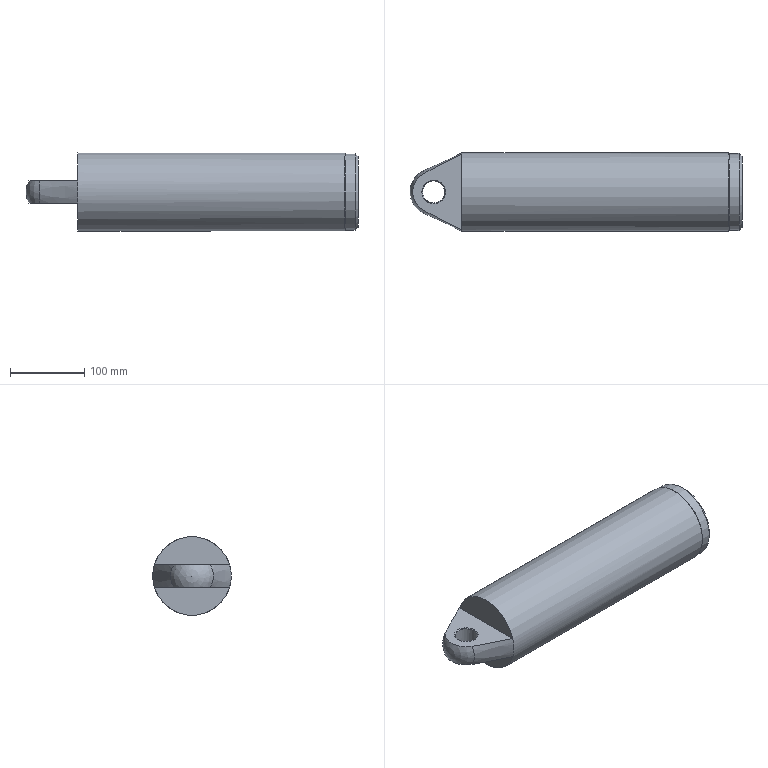Part | NX | features 侧推千斤顶缸 2 | 1 solid | 17 faces | box 448 x 106 x 106 mm | volume 2799935 mm3 | cone 6 | plane 6 | cylinder 4 | sphere 1 | commonest cylinder face diameters 30 x1 50.16 x1 104 x1 106 x1
STEP:
#1=CARTESIAN_POINT('',(0.,-50.833,-15.));
#2=VERTEX_POINT('',#1);
#3=CARTESIAN_POINT('',(0.,-50.833,15.));
#4=VERTEX_POINT('',#3);
#5=CARTESIAN_POINT('',(0.,0.,0.));
#6=DIRECTION('',(-1.,0.,0.));
#7=DIRECTION('',(0.,-1.,0.));
#8=AXIS2_PLACEMENT_3D('',#5,#6,#7);
#9=CIRCLE('',#8,53.);
#10=EDGE_CURVE('',#2,#4,#9,.T.);
#11=ORIENTED_EDGE('',*,*,#10,.T.);
#12=CARTESIAN_POINT('',(-51.511,-24.829,15.));
#13=VERTEX_POINT('',#12);
#14=CARTESIAN_POINT('',(0.,-50.833,15.));
#15=CARTESIAN_POINT('',(-8.652,-46.632,15.));
#16=CARTESIAN_POINT('',(-25.92,-38.162,15.));
#17=CARTESIAN_POINT('',(-43.068,-29.423,15.));
#18=CARTESIAN_POINT('',(-51.511,-24.829,15.));
#19=B_SPLINE_CURVE_WITH_KNOTS('',3,(#14,#15,#16,#17,#18),.UNSPECIFIED.,.F.,.F.,(4,1,4),(0.07837,0.1072,0.1361),.UNSPECIFIED.);
#20=EDGE_CURVE('',#4,#13,#19,.T.);
#21=ORIENTED_EDGE('',*,*,#20,.T.);
#22=CARTESIAN_POINT('',(-51.511,-24.829,-15.));
#23=VERTEX_POINT('',#22);
#24=CARTESIAN_POINT('',(-51.511,0.,0.));
#25=DIRECTION('',(-1.,0.,0.));
#26=DIRECTION('',(0.,-1.,0.));
#27=AXIS2_PLACEMENT_3D('',#24,#25,#26);
#28=CIRCLE('',#27,29.008);
#29=EDGE_CURVE('',#23,#13,#28,.T.);
#30=ORIENTED_EDGE('',*,*,#29,.F.);
#31=CARTESIAN_POINT('',(-51.511,-24.829,-15.));
#32=CARTESIAN_POINT('',(-43.068,-29.423,-15.));
#33=CARTESIAN_POINT('',(-25.924,-38.16,-15.));
#34=CARTESIAN_POINT('',(-8.652,-46.631,-15.));
#35=CARTESIAN_POINT('',(0.,-50.833,-15.));
#36=B_SPLINE_CURVE_WITH_KNOTS('',3,(#31,#32,#33,#34,#35),.UNSPECIFIED.,.F.,.F.,(4,1,4),(0.2163,0.2453,0.2742),.UNSPECIFIED.);
#37=EDGE_CURVE('',#23,#2,#36,.T.);
#38=ORIENTED_EDGE('',*,*,#37,.T.);
#39=EDGE_LOOP('',(#11,#21,#30,#38));
#40=FACE_BOUND('',#39,.T.);
#41=CARTESIAN_POINT('',(0.,0.,0.));
#42=DIRECTION('',(1.,0.,0.));
#43=DIRECTION('',(0.,1.,0.));
#44=AXIS2_PLACEMENT_3D('',#41,#42,#43);
#45=CONICAL_SURFACE('',#44,53.,0.4359);
#46=ADVANCED_FACE('',(#40),#45,.T.);
#47=CARTESIAN_POINT('',(-51.511,24.829,15.));
#48=VERTEX_POINT('',#47);
#49=CARTESIAN_POINT('',(-51.511,24.829,-15.));
#50=VERTEX_POINT('',#49);
#51=CARTESIAN_POINT('',(-51.511,0.,0.));
#52=DIRECTION('',(-1.,0.,0.));
#53=DIRECTION('',(0.,-1.,0.));
#54=AXIS2_PLACEMENT_3D('',#51,#52,#53);
#55=CIRCLE('',#54,29.008);
#56=EDGE_CURVE('',#48,#50,#55,.T.);
#57=ORIENTED_EDGE('',*,*,#56,.F.);
#58=CARTESIAN_POINT('',(0.,50.833,15.));
#59=VERTEX_POINT('',#58);
#60=CARTESIAN_POINT('',(-51.511,24.829,15.));
#61=CARTESIAN_POINT('',(-43.068,29.423,15.));
#62=CARTESIAN_POINT('',(-25.924,38.16,15.));
#63=CARTESIAN_POINT('',(-8.652,46.631,15.));
#64=CARTESIAN_POINT('',(0.,50.833,15.));
#65=B_SPLINE_CURVE_WITH_KNOTS('',3,(#60,#61,#62,#63,#64),.UNSPECIFIED.,.F.,.F.,(4,1,4),(0.2163,0.2453,0.2742),.UNSPECIFIED.);
#66=EDGE_CURVE('',#48,#59,#65,.T.);
#67=ORIENTED_EDGE('',*,*,#66,.T.);
#68=CARTESIAN_POINT('',(0.,50.833,-15.));
#69=VERTEX_POINT('',#68);
#70=CARTESIAN_POINT('',(0.,0.,0.));
#71=DIRECTION('',(-1.,0.,0.));
#72=DIRECTION('',(0.,-1.,0.));
#73=AXIS2_PLACEMENT_3D('',#70,#71,#72);
#74=CIRCLE('',#73,53.);
#75=EDGE_CURVE('',#59,#69,#74,.T.);
#76=ORIENTED_EDGE('',*,*,#75,.T.);
#77=CARTESIAN_POINT('',(0.,50.833,-15.));
#78=CARTESIAN_POINT('',(-8.652,46.632,-15.));
#79=CARTESIAN_POINT('',(-25.92,38.162,-15.));
#80=CARTESIAN_POINT('',(-43.068,29.423,-15.));
#81=CARTESIAN_POINT('',(-51.511,24.829,-15.));
#82=B_SPLINE_CURVE_WITH_KNOTS('',3,(#77,#78,#79,#80,#81),.UNSPECIFIED.,.F.,.F.,(4,1,4),(0.07837,0.1072,0.1361),.UNSPECIFIED.);
#83=EDGE_CURVE('',#69,#50,#82,.T.);
#84=ORIENTED_EDGE('',*,*,#83,.T.);
#85=EDGE_LOOP('',(#57,#67,#76,#84));
#86=FACE_BOUND('',#85,.T.);
#87=CARTESIAN_POINT('',(0.,0.,0.));
#88=DIRECTION('',(1.,0.,0.));
#89=DIRECTION('',(0.,1.,0.));
#90=AXIS2_PLACEMENT_3D('',#87,#88,#89);
#91=CONICAL_SURFACE('',#90,53.,0.4359);
#92=ADVANCED_FACE('',(#86),#91,.T.);
#93=ORIENTED_EDGE('',*,*,#29,.T.);
#94=CARTESIAN_POINT('',(-38.,0.,15.));
#95=DIRECTION('',(0.,0.,-1.));
#96=DIRECTION('',(0.,1.,0.));
#97=AXIS2_PLACEMENT_3D('',#94,#95,#96);
#98=CIRCLE('',#97,28.267);
#99=EDGE_CURVE('',#13,#48,#98,.T.);
#100=ORIENTED_EDGE('',*,*,#99,.T.);
#101=ORIENTED_EDGE('',*,*,#56,.T.);
#102=CARTESIAN_POINT('',(-38.,0.,-15.));
#103=DIRECTION('',(0.,0.,1.));
#104=DIRECTION('',(0.,-1.,0.));
#105=AXIS2_PLACEMENT_3D('',#102,#103,#104);
#106=CIRCLE('',#105,28.267);
#107=EDGE_CURVE('',#50,#23,#106,.T.);
#108=ORIENTED_EDGE('',*,*,#107,.T.);
#109=EDGE_LOOP('',(#93,#100,#101,#108));
#110=FACE_BOUND('',#109,.T.);
#111=CARTESIAN_POINT('',(-38.,0.,0.));
#112=DIRECTION('',(-1.,0.,0.));
#113=DIRECTION('',(0.,1.,0.));
#114=AXIS2_PLACEMENT_3D('',#111,#112,#113);
#115=SPHERICAL_SURFACE('',#114,32.);
#116=ADVANCED_FACE('',(#110),#115,.T.);
#117=CARTESIAN_POINT('',(378.,0.,-25.08));
#118=VERTEX_POINT('',#117);
#119=CARTESIAN_POINT('',(378.,0.,0.));
#120=DIRECTION('',(1.,0.,0.));
#121=DIRECTION('',(0.,0.,-1.));
#122=AXIS2_PLACEMENT_3D('',#119,#120,#121);
#123=CIRCLE('',#122,25.08);
#124=EDGE_CURVE('',#118,#118,#123,.T.);
#125=ORIENTED_EDGE('',*,*,#124,.F.);
#126=EDGE_LOOP('',(#125));
#127=FACE_BOUND('',#126,.T.);
#128=CARTESIAN_POINT('',(378.,-48.,0.));
#129=VERTEX_POINT('',#128);
#130=CARTESIAN_POINT('',(378.,0.,0.));
#131=DIRECTION('',(-1.,0.,0.));
#132=DIRECTION('',(0.,-1.,0.));
#133=AXIS2_PLACEMENT_3D('',#130,#131,#132);
#134=CIRCLE('',#133,48.);
#135=EDGE_CURVE('',#129,#129,#134,.T.);
#136=ORIENTED_EDGE('',*,*,#135,.F.);
#137=EDGE_LOOP('',(#136));
#138=FACE_BOUND('',#137,.T.);
#139=CARTESIAN_POINT('',(378.,48.,0.));
#140=DIRECTION('',(-1.,0.,0.));
#141=DIRECTION('',(0.,-1.,0.));
#142=AXIS2_PLACEMENT_3D('',#139,#140,#141);
#143=PLANE('',#142);
#144=ADVANCED_FACE('',(#127,#138),#143,.F.);
#145=CARTESIAN_POINT('',(374.,-52.,0.));
#146=VERTEX_POINT('',#145);
#147=CARTESIAN_POINT('',(374.,0.,0.));
#148=DIRECTION('',(-1.,0.,0.));
#149=DIRECTION('',(0.,-1.,0.));
#150=AXIS2_PLACEMENT_3D('',#147,#148,#149);
#151=CIRCLE('',#150,52.);
#152=EDGE_CURVE('',#146,#146,#151,.T.);
#153=ORIENTED_EDGE('',*,*,#152,.F.);
#154=EDGE_LOOP('',(#153));
#155=FACE_BOUND('',#154,.T.);
#156=ORIENTED_EDGE('',*,*,#135,.T.);
#157=EDGE_LOOP('',(#156));
#158=FACE_BOUND('',#157,.T.);
#159=CARTESIAN_POINT('',(378.,0.,0.));
#160=DIRECTION('',(-1.,0.,0.));
#161=DIRECTION('',(0.,-1.,0.));
#162=AXIS2_PLACEMENT_3D('',#159,#160,#161);
#163=CONICAL_SURFACE('',#162,48.,0.7854);
#164=ADVANCED_FACE('',(#155,#158),#163,.T.);
#165=CARTESIAN_POINT('',(361.,-52.,0.));
#166=VERTEX_POINT('',#165);
#167=CARTESIAN_POINT('',(361.,0.,0.));
#168=DIRECTION('',(-1.,0.,0.));
#169=DIRECTION('',(0.,-1.,0.));
#170=AXIS2_PLACEMENT_3D('',#167,#168,#169);
#171=CIRCLE('',#170,52.);
#172=EDGE_CURVE('',#166,#166,#171,.T.);
#173=ORIENTED_EDGE('',*,*,#172,.F.);
#174=EDGE_LOOP('',(#173));
#175=FACE_BOUND('',#174,.T.);
#176=ORIENTED_EDGE('',*,*,#152,.T.);
#177=EDGE_LOOP('',(#176));
#178=FACE_BOUND('',#177,.T.);
#179=CARTESIAN_POINT('',(0.,0.,0.));
#180=DIRECTION('',(-1.,0.,0.));
#181=DIRECTION('',(0.,-1.,0.));
#182=AXIS2_PLACEMENT_3D('',#179,#180,#181);
#183=CYLINDRICAL_SURFACE('',#182,52.);
#184=ADVANCED_FACE('',(#175,#178),#183,.T.);
#185=CARTESIAN_POINT('',(360.,-53.,0.));
#186=VERTEX_POINT('',#185);
#187=CARTESIAN_POINT('',(360.,0.,0.));
#188=DIRECTION('',(-1.,0.,0.));
#189=DIRECTION('',(0.,-1.,0.));
#190=AXIS2_PLACEMENT_3D('',#187,#188,#189);
#191=CIRCLE('',#190,53.);
#192=EDGE_CURVE('',#186,#186,#191,.T.);
#193=ORIENTED_EDGE('',*,*,#192,.F.);
#194=EDGE_LOOP('',(#193));
#195=FACE_BOUND('',#194,.T.);
#196=ORIENTED_EDGE('',*,*,#172,.T.);
#197=EDGE_LOOP('',(#196));
#198=FACE_BOUND('',#197,.T.);
#199=CARTESIAN_POINT('',(361.,0.,0.));
#200=DIRECTION('',(-1.,0.,0.));
#201=DIRECTION('',(0.,-1.,0.));
#202=AXIS2_PLACEMENT_3D('',#199,#200,#201);
#203=CONICAL_SURFACE('',#202,52.,0.7854);
#204=ADVANCED_FACE('',(#195,#198),#203,.T.);
#205=CARTESIAN_POINT('',(0.,0.,0.));
#206=DIRECTION('',(-1.,0.,0.));
#207=DIRECTION('',(0.,-1.,0.));
#208=AXIS2_PLACEMENT_3D('',#205,#206,#207);
#209=CIRCLE('',#208,53.);
#210=EDGE_CURVE('',#69,#2,#209,.T.);
#211=ORIENTED_EDGE('',*,*,#210,.F.);
#212=ORIENTED_EDGE('',*,*,#75,.F.);
#213=CARTESIAN_POINT('',(0.,0.,0.));
#214=DIRECTION('',(-1.,0.,0.));
#215=DIRECTION('',(0.,-1.,0.));
#216=AXIS2_PLACEMENT_3D('',#213,#214,#215);
#217=CIRCLE('',#216,53.);
#218=EDGE_CURVE('',#4,#59,#217,.T.);
#219=ORIENTED_EDGE('',*,*,#218,.F.);
#220=ORIENTED_EDGE('',*,*,#10,.F.);
#221=EDGE_LOOP('',(#211,#212,#219,#220));
#222=FACE_BOUND('',#221,.T.);
#223=ORIENTED_EDGE('',*,*,#192,.T.);
#224=EDGE_LOOP('',(#223));
#225=FACE_BOUND('',#224,.T.);
#226=CARTESIAN_POINT('',(0.,0.,0.));
#227=DIRECTION('',(-1.,0.,0.));
#228=DIRECTION('',(0.,-1.,0.));
#229=AXIS2_PLACEMENT_3D('',#226,#227,#228);
#230=CYLINDRICAL_SURFACE('',#229,53.);
#231=ADVANCED_FACE('',(#222,#225),#230,.T.);
#232=CARTESIAN_POINT('',(48.8,0.,-25.08));
#233=VERTEX_POINT('',#232);
#234=CARTESIAN_POINT('',(48.8,0.,0.));
#235=DIRECTION('',(1.,0.,0.));
#236=DIRECTION('',(0.,0.,-1.));
#237=AXIS2_PLACEMENT_3D('',#234,#235,#236);
#238=CIRCLE('',#237,25.08);
#239=EDGE_CURVE('',#233,#233,#238,.T.);
#240=ORIENTED_EDGE('',*,*,#239,.F.);
#241=EDGE_LOOP('',(#240));
#242=FACE_BOUND('',#241,.T.);
#243=ORIENTED_EDGE('',*,*,#124,.T.);
#244=EDGE_LOOP('',(#243));
#245=FACE_BOUND('',#244,.T.);
#246=CARTESIAN_POINT('',(48.8,0.,0.));
#247=DIRECTION('',(1.,0.,0.));
#248=DIRECTION('',(0.,0.,-1.));
#249=AXIS2_PLACEMENT_3D('',#246,#247,#248);
#250=CYLINDRICAL_SURFACE('',#249,25.08);
#251=ADVANCED_FACE('',(#242,#245),#250,.F.);
#252=ORIENTED_EDGE('',*,*,#239,.T.);
#253=EDGE_LOOP('',(#252));
#254=FACE_BOUND('',#253,.T.);
#255=CARTESIAN_POINT('',(48.8,0.,0.));
#256=DIRECTION('',(1.,0.,0.));
#257=DIRECTION('',(0.,0.,-1.));
#258=AXIS2_PLACEMENT_3D('',#255,#256,#257);
#259=PLANE('',#258);
#260=ADVANCED_FACE('',(#254),#259,.T.);
#261=CARTESIAN_POINT('',(-23.,0.,-14.));
#262=VERTEX_POINT('',#261);
#263=CARTESIAN_POINT('',(-38.,0.,-14.));
#264=DIRECTION('',(0.,0.,1.));
#265=DIRECTION('',(1.,0.,0.));
#266=AXIS2_PLACEMENT_3D('',#263,#264,#265);
#267=CIRCLE('',#266,15.);
#268=EDGE_CURVE('',#262,#262,#267,.F.);
#269=ORIENTED_EDGE('',*,*,#268,.T.);
#270=EDGE_LOOP('',(#269));
#271=FACE_BOUND('',#270,.T.);
#272=CARTESIAN_POINT('',(-53.,0.,14.));
#273=VERTEX_POINT('',#272);
#274=CARTESIAN_POINT('',(-38.,0.,14.));
#275=DIRECTION('',(0.,0.,-1.));
#276=DIRECTION('',(-1.,0.,0.));
#277=AXIS2_PLACEMENT_3D('',#274,#275,#276);
#278=CIRCLE('',#277,15.);
#279=EDGE_CURVE('',#273,#273,#278,.F.);
#280=ORIENTED_EDGE('',*,*,#279,.T.);
#281=EDGE_LOOP('',(#280));
#282=FACE_BOUND('',#281,.T.);
#283=CARTESIAN_POINT('',(-38.,0.,-50.));
#284=DIRECTION('',(0.,0.,1.));
#285=DIRECTION('',(1.,0.,0.));
#286=AXIS2_PLACEMENT_3D('',#283,#284,#285);
#287=CYLINDRICAL_SURFACE('',#286,15.);
#288=ADVANCED_FACE('',(#271,#282),#287,.F.);
#289=ORIENTED_EDGE('',*,*,#210,.T.);
#290=CARTESIAN_POINT('',(0.,53.,-15.));
#291=DIRECTION('',(0.,-1.,0.));
#292=VECTOR('',#291,1000.);
#293=LINE('',#290,#292);
#294=EDGE_CURVE('',#69,#2,#293,.T.);
#295=ORIENTED_EDGE('',*,*,#294,.F.);
#296=EDGE_LOOP('',(#289,#295));
#297=FACE_BOUND('',#296,.T.);
#298=CARTESIAN_POINT('',(0.,-53.,-55.37));
#299=DIRECTION('',(-1.,0.,0.));
#300=DIRECTION('',(0.,0.,1.));
#301=AXIS2_PLACEMENT_3D('',#298,#299,#300);
#302=PLANE('',#301);
#303=ADVANCED_FACE('',(#297),#302,.T.);
#304=CARTESIAN_POINT('',(-38.,-16.,-15.));
#305=VERTEX_POINT('',#304);
#306=CARTESIAN_POINT('',(-38.,0.,-15.));
#307=DIRECTION('',(0.,0.,1.));
#308=DIRECTION('',(0.,-1.,0.));
#309=AXIS2_PLACEMENT_3D('',#306,#307,#308);
#310=CIRCLE('',#309,16.);
#311=EDGE_CURVE('',#305,#305,#310,.T.);
#312=ORIENTED_EDGE('',*,*,#311,.T.);
#313=EDGE_LOOP('',(#312));
#314=FACE_BOUND('',#313,.T.);
#315=ORIENTED_EDGE('',*,*,#294,.T.);
#316=ORIENTED_EDGE('',*,*,#37,.F.);
#317=ORIENTED_EDGE('',*,*,#107,.F.);
#318=ORIENTED_EDGE('',*,*,#83,.F.);
#319=EDGE_LOOP('',(#315,#316,#317,#318));
#320=FACE_BOUND('',#319,.T.);
#321=CARTESIAN_POINT('',(-100.,53.,-15.));
#322=DIRECTION('',(0.,0.,1.));
#323=DIRECTION('',(0.,-1.,0.));
#324=AXIS2_PLACEMENT_3D('',#321,#322,#323);
#325=PLANE('',#324);
#326=ADVANCED_FACE('',(#314,#320),#325,.F.);
#327=CARTESIAN_POINT('',(0.,53.,15.));
#328=DIRECTION('',(0.,1.,0.));
#329=VECTOR('',#328,1000.);
#330=LINE('',#327,#329);
#331=EDGE_CURVE('',#4,#59,#330,.T.);
#332=ORIENTED_EDGE('',*,*,#331,.F.);
#333=ORIENTED_EDGE('',*,*,#218,.T.);
#334=EDGE_LOOP('',(#332,#333));
#335=FACE_BOUND('',#334,.T.);
#336=CARTESIAN_POINT('',(0.,-53.,55.188));
#337=DIRECTION('',(1.,0.,0.));
#338=DIRECTION('',(0.,0.,-1.));
#339=AXIS2_PLACEMENT_3D('',#336,#337,#338);
#340=PLANE('',#339);
#341=ADVANCED_FACE('',(#335),#340,.F.);
#342=CARTESIAN_POINT('',(-38.,16.,15.));
#343=VERTEX_POINT('',#342);
#344=CARTESIAN_POINT('',(-38.,0.,15.));
#345=DIRECTION('',(0.,0.,-1.));
#346=DIRECTION('',(0.,1.,0.));
#347=AXIS2_PLACEMENT_3D('',#344,#345,#346);
#348=CIRCLE('',#347,16.);
#349=EDGE_CURVE('',#343,#343,#348,.T.);
#350=ORIENTED_EDGE('',*,*,#349,.T.);
#351=EDGE_LOOP('',(#350));
#352=FACE_BOUND('',#351,.T.);
#353=ORIENTED_EDGE('',*,*,#331,.T.);
#354=ORIENTED_EDGE('',*,*,#66,.F.);
#355=ORIENTED_EDGE('',*,*,#99,.F.);
#356=ORIENTED_EDGE('',*,*,#20,.F.);
#357=EDGE_LOOP('',(#353,#354,#355,#356));
#358=FACE_BOUND('',#357,.T.);
#359=CARTESIAN_POINT('',(-100.,53.,15.));
#360=DIRECTION('',(0.,0.,-1.));
#361=DIRECTION('',(0.,1.,0.));
#362=AXIS2_PLACEMENT_3D('',#359,#360,#361);
#363=PLANE('',#362);
#364=ADVANCED_FACE('',(#352,#358),#363,.F.);
#365=ORIENTED_EDGE('',*,*,#311,.F.);
#366=EDGE_LOOP('',(#365));
#367=FACE_BOUND('',#366,.T.);
#368=ORIENTED_EDGE('',*,*,#268,.F.);
#369=EDGE_LOOP('',(#368));
#370=FACE_BOUND('',#369,.T.);
#371=CARTESIAN_POINT('',(-38.,0.,-14.));
#372=DIRECTION('',(0.,0.,-1.));
#373=DIRECTION('',(-1.,0.,0.));
#374=AXIS2_PLACEMENT_3D('',#371,#372,#373);
#375=CONICAL_SURFACE('',#374,15.,0.7854);
#376=ADVANCED_FACE('',(#367,#370),#375,.F.);
#377=ORIENTED_EDGE('',*,*,#349,.F.);
#378=EDGE_LOOP('',(#377));
#379=FACE_BOUND('',#378,.T.);
#380=ORIENTED_EDGE('',*,*,#279,.F.);
#381=EDGE_LOOP('',(#380));
#382=FACE_BOUND('',#381,.T.);
#383=CARTESIAN_POINT('',(-38.,0.,14.));
#384=DIRECTION('',(0.,0.,1.));
#385=DIRECTION('',(1.,0.,0.));
#386=AXIS2_PLACEMENT_3D('',#383,#384,#385);
#387=CONICAL_SURFACE('',#386,15.,0.7854);
#388=ADVANCED_FACE('',(#379,#382),#387,.F.);
#389=CLOSED_SHELL('',(#46,#92,#116,#144,#164,#184,#204,#231,#251,#260,#288,#303,#326,#341,#364,#376,#388));
#390=MANIFOLD_SOLID_BREP('',#389);
#391=(LENGTH_UNIT()NAMED_UNIT(*)SI_UNIT(.MILLI.,.METRE.));
#392=UNCERTAINTY_MEASURE_WITH_UNIT(LENGTH_MEASURE(0.0508),#391,'','');
#393=(NAMED_UNIT(*)PLANE_ANGLE_UNIT()SI_UNIT($,.RADIAN.));
#394=(NAMED_UNIT(*)SI_UNIT($,.STERADIAN.)SOLID_ANGLE_UNIT());
#395=(GEOMETRIC_REPRESENTATION_CONTEXT(3)GLOBAL_UNCERTAINTY_ASSIGNED_CONTEXT((#392))GLOBAL_UNIT_ASSIGNED_CONTEXT((#391,#393,#394))REPRESENTATION_CONTEXT('',''));
#396=ADVANCED_BREP_SHAPE_REPRESENTATION('',(#390),#395);